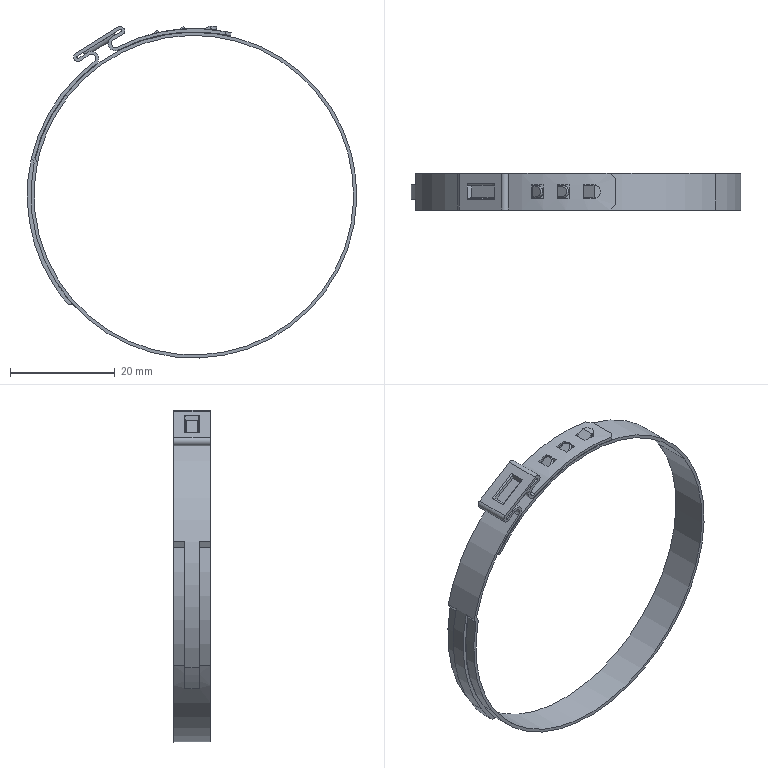Part | SolidWorks | features BaseBody 1 | 1 solid | 101 faces | box 63 x 7 x 63.493 mm | volume 1084 mm3 | plane 56 | cylinder 37 | spline 8 | commonest cylinder face diameters 62.3 x6 2.8 x5 61.1 x5 1.7 x4 1.6 x3 63.7 x3